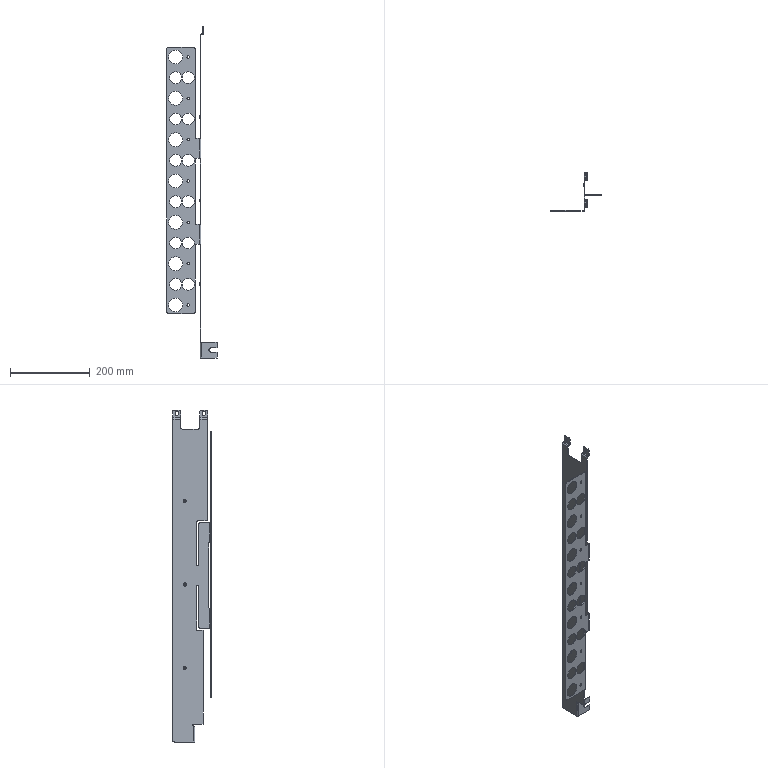Part | STEP file | 64524283 | 1 solid | 202 faces | box 126.2 x 96.5 x 835.25 mm | volume 152034 mm3 | cylinder 107 | plane 83 | torus 12 | commonest cylinder face diameters 30 x24 8 x21 6.5 x14 35 x14 3 x7 6 x7